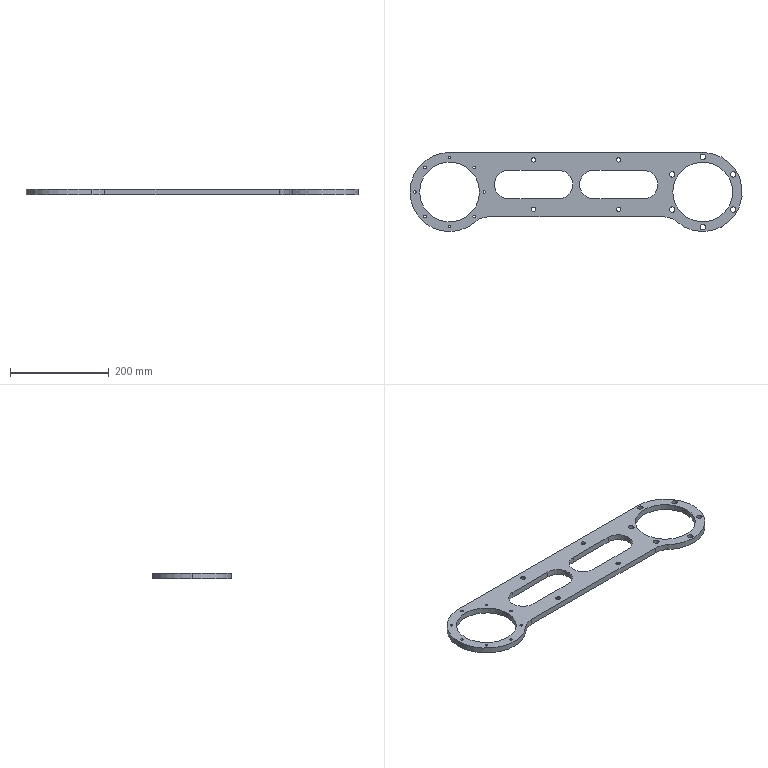Part | SolidWorks | features ICE 5, Extrusion 1, HoleWzd 1 | 1 solid | 71 faces | box 672 x 160 x 12 mm | volume 577660 mm3 | cylinder 59 | plane 12 | commonest cylinder face diameters 5 x16 11 x12 9 x8 15 x8 58 x6 121 x4